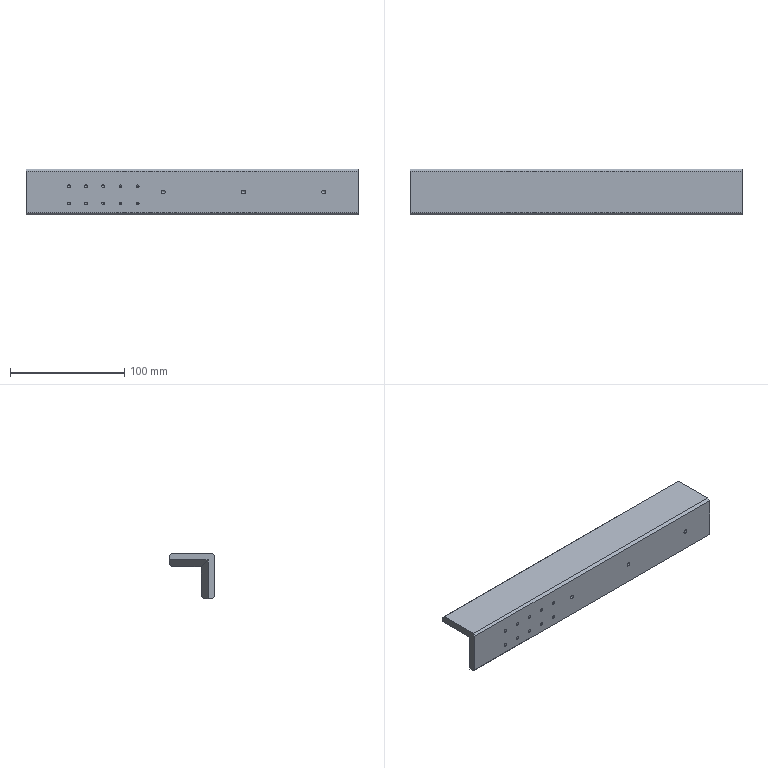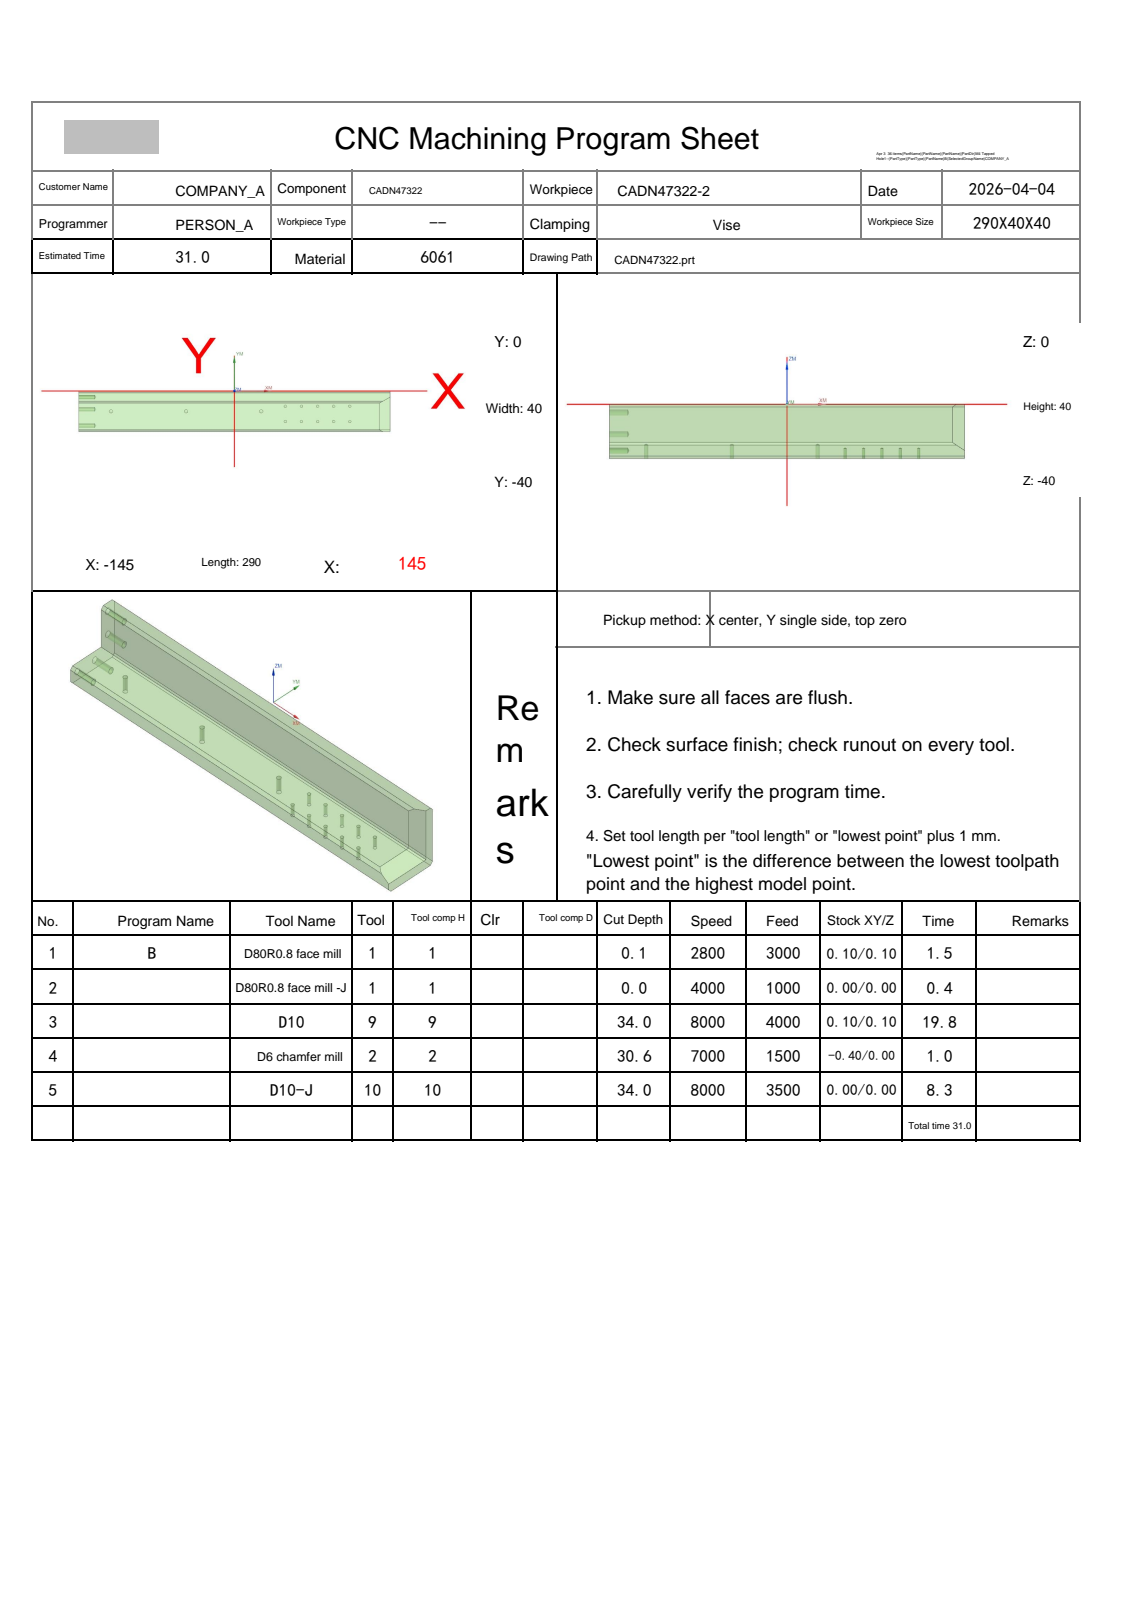NC program | NX | posted by the shop | part box 290 x 40 x 40 mm
Lines 1 to 108 of 6219:
%
O0001
(Machine time: 32.95 MIN)
(===Total Tool:4===)
(T1=D80R0.8 face mill D=80.  R=0.8  D-  H01 Z=0.    )
(T9=D10     D=10.  R=0.   D-  H09 Z=-34.  )
(T2=D6 chamfer mill   D=6.   R=0.   D-  H02 Z=-30.6 )
(T10=D10-J  D=10.  R=0.   D10 H10 Z=-34.  )
G80 G90 G17 G49 G40
G91 G28 Z0
M01
N1 T01 M06
(D80R0.8 face mill  D=80. R=0.8 H=01 ce=0.10 di=0.10)
G00 G90 G54 X-197.097 Y-20. M03 S2800
G43 H01 Z20.
M08
Z6.011
G01 Z4.011 F3000.
X-185.097
X185.097
X197.097
Z6.011
G00 X-197.097
Z5.522
G01 Z3.522
X-185.097
X185.097
X197.097
Z5.522
G00 X-197.097
Z5.033
G01 Z3.033
X-185.097
X185.097
X197.097
Z5.033
G00 X-197.097
Z4.544
G01 Z2.544
X-185.097
X185.097
X197.097
Z4.544
G00 Z20.
X-197.097
Z4.056
G01 Z2.056
X-185.097
X185.097
X197.097
Z4.056
G00 Z20.
X-197.097
Z3.567
G01 Z1.567
X-185.097
X185.097
X197.097
Z3.567
G00 Z20.
X-197.097
Z3.078
G01 Z1.078
X-185.097
X185.097
X197.097
Z3.078
G00 Z20.
X-197.097
Z2.589
G01 Z.589
X-185.097
X185.097
X197.097
Z2.589
G00 Z20.
X-197.097
Z2.1
G01 Z.1
X-185.097
X185.097
X197.097
Z2.1
G00 Z20.
G91 G28 Z0.0
M05
M09
G91 G28 Z0.0
M01
N2 T01 M06
(D80R0.8 face mill-J  D=80. R=0.8 H=01 ce=0.00 di=0.00)
G00 G90 G54 X-196.999 Y-20. M03 S4000
G43 H01 Z20.
M08
Z2.
G01 Z0.0 F1000.
X-184.999
X184.999
X196.999
Z2.
G00 Z20.
G91 G28 Z0.0
M05
M09
G91 G28 Z0.0
M01